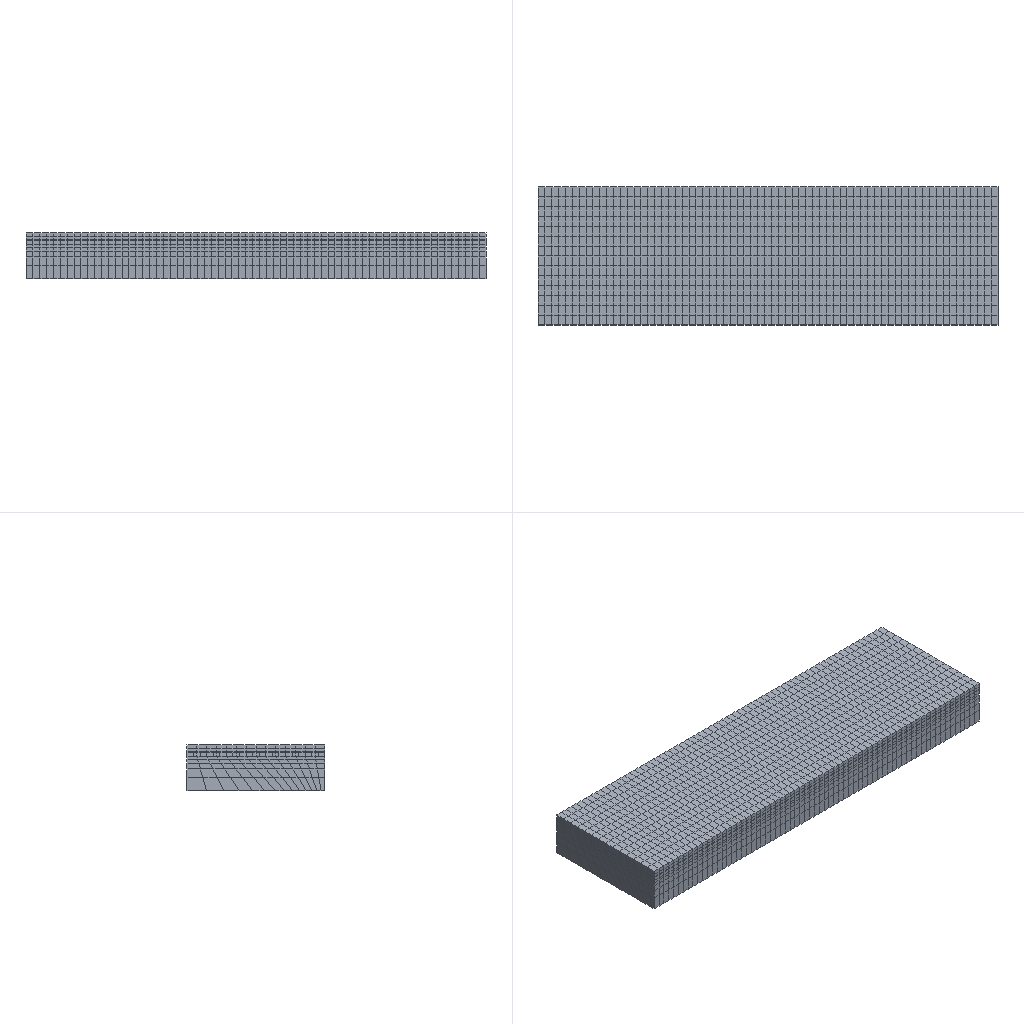Simulation study | abaqus
Set-up summary:
category,name,step,type,value,unit,region
solver,abaqus
solver,version,,,Abaqus/Explicit 2020
units,not stated in the deck,,not stated
analysis,deck,,transient,transient
load_step,Step-1,Step-1,transient
load_step,requested,,,1
mesh,nodes,,,12922
mesh,elements,,,9772
element_type,R3D3,,rigid,228
element_type,R3D4,,rigid,633
element_type,C3D8R,,solid,1407
element_type,EC3D8R,,solid,7504
load,load commands in deck,,count,1
bc,support commands in deck,,count,10
material,BING,,in results
material,WATER,,in results
check,setup vs results,,match,"per instance, exact: element labels, types and connectivity; labels of the nodes the elements use; coordinates of those nodes at SINGLE_PRECISION in 2 of 3 instance(s)"
Abaqus input file, long lists of numbers shortened:
*Heading
** Job name: Job-1 Model name: Model-1
** Generated by: Abaqus/CAE 2020
*Preprint, echo=NO, model=NO, history=NO, contact=NO
**
** PARTS
**
*Part, name=bing
*Node
      1,           0.,       -3000.,         900.
      2,       10000.,       -3000.,         900.
** (2990 more lines like these left out)
*Element, type=C3D8R
  1,  292,  617, 1013,  281,    1,   17,  148,    4
  2,  617,  618, 1014, 1013,   17,   18,  147,  148
** (1405 more lines like these left out)
*Nset, nset=Set-1, generate
    1,  2992,     1
*Elset, elset=Set-1, generate
    1,  1407,     1
** Section: bing
*Solid Section, elset=Set-1, material=bing
,
*End Part
**
*Part, name=oula
*Node
      1,       10000.,           0.,         750.
      2,       10000.,       -3000.,         750.
** (9178 more lines like these left out)
*Element, type=EC3D8R
   1,  212, 1143, 4033,  615,    1,   13,  511,   46
   2, 1143, 1144, 4034, 4033,   13,   14,  512,  511
** (7502 more lines like these left out)
*Nset, nset=Set-1, generate
    1,  9180,     1
*Elset, elset=Set-1, generate
    1,  7504,     1
** Section: oula
*Eulerian Section, elset=Set-1
water, water-1
*Surface, type=EULERIAN MATERIAL, name=water-1
water-1
*End Part
**
*Part, name=work
*Node
      1,    2.375,   6757.633,   37190.746
      2,    2.375,   6757.633,   40618.258
** (747 more lines like these left out)
*Element, type=R3D4
 1,  1, 21, 64,  4
 2, 21, 22, 63, 64
** (631 more lines like these left out)
*Element, type=R3D3
369,  4, 65,  5
370, 71, 59, 58
** (226 more lines like these left out)
*Node
    750,    2.375,   6959.508,   38910.039
*Nset, nset=work-RefPt_, internal
750,
*Elset, elset=work, generate
   1,  861,    1
*End Part
**
**
** ASSEMBLY
**
*Assembly, name=Assembly
**
*Instance, name=work-1, part=work
37076.822, -1497.625, -5616.383
37076.822, -1497.625, -5616.383, 37077.399, -1498.203, -5616.96,         120.
*End Instance
**
*Instance, name=oula-1, part=oula
          0.,           0.,         250.
*End Instance
**
*Instance, name=bing-1, part=bing
          0.,           0.,         100.
*End Instance
**
*Nset, nset=Set-1, instance=oula-1
    1,    2,    3,    4,    5,    6,    7,    8,   13,   14,   15,   16,   17,   18,   19,   20
   21,   22,   23,   24,   25,   26,   27,   28,   29,   30,   31,   32,   33,   34,   35,   36
** (381 more lines like these left out)
*Elset, elset=Set-1, instance=oula-1, generate
    1,  4690,     1
*Nset, nset=Set-2, instance=bing-1
   1,   2,   3,   4,   5,   6,   9,  12,  13,  14,  15,  16,  17,  18,  19,  20
  21,  22,  23,  24,  25,  26,  27,  28,  29,  30,  31,  32,  33,  34,  35,  36
** (18 more lines like these left out)
*Elset, elset=Set-2, instance=bing-1
    1,    2,    3,    4,    5,    6,    7,    8,    9,   10,   11,   12,   13,   14,   15,   16
   17,   18,   19,   20,   21,   22,   23,   24,   25,   26,   27,   28,   29,   30,   31,   32
** (8 more lines like these left out)
*Nset, nset=Set-3, instance=oula-1
    1,    2,    3,    4,    5,    6,    7,    8,    9,   10,   11,   12,   26,   27,   28,   29
   43,   44,   45,   46,   60,   61,   62,   63,   77,   78,   79,   80,   81,   82,   83,   84
** (75 more lines like these left out)
*Elset, elset=Set-3, instance=oula-1
    1,   14,   15,   28,   29,   42,   43,   56,   57,   70,   71,   84,   85,   98,   99,  112
  113,  126,  127,  140,  141,  154,  155,  168,  169,  182,  183,  196,  197,  210,  211,  224
** (65 more lines like these left out)
*Nset, nset=Set-4, instance=oula-1
    3,    4,    6,    7,   30,   31,   32,   33,   34,   35,   36,   37,   38,   39,   40,   41
   42,   64,   65,   66,   67,   68,   69,   70,   71,   72,   73,   74,   75,   76,   81,   82
** (62 more lines like these left out)
*Elset, elset=Set-4, instance=oula-1
   57,   58,   59,   60,   61,   62,   63,   64,   65,   66,   67,   68,   69,   70,  127,  128
  129,  130,  131,  132,  133,  134,  135,  136,  137,  138,  139,  140,  197,  198,  199,  200
** (57 more lines like these left out)
*Nset, nset=Set-5, instance=oula-1
   1,   2,   3,   4,  13,  14,  15,  16,  17,  18,  19,  20,  21,  22,  23,  24
  25,  26,  27,  28,  29,  30,  31,  32,  33,  34,  35,  36,  37,  38,  39,  40
** (4 more lines like these left out)
*Elset, elset=Set-5, instance=oula-1, generate
  1,  70,   1
*Nset, nset=Set-6, instance=work-1
 750,
*Rigid Body, ref node=work-1.work-RefPt_, elset=work-1.work
*End Assembly
**
** MATERIALS
**
*Material, name=bing
*Brittle Cracking
100.,  0.
250., 0.1
*Brittle Shear
1.,  0.
0., 0.1
*Brittle Failure
1.,
*Density
 9.2e-10,
*Elastic
1000., 0.3
*Material, name=water
*Density
 1e-09,
*Eos, type=USUP
1483.,0.,0.
*Viscosity
 0.01,
**
** INTERACTION PROPERTIES
**
*Surface Interaction, name=IntProp-1
*Friction
 0.2,
*Surface Behavior, pressure-overclosure=HARD
**
** PREDEFINED FIELDS
**
** Name: Predefined Field-1   Type: Material assignment
*Initial Conditions, type=VOLUME FRACTION
Set-1, oula-1.water-1, 1.
** ----------------------------------------------------------------
**
** STEP: Step-1
**
*Step, name=Step-1, nlgeom=YES
*Dynamic, Explicit
, 1.
*Bulk Viscosity
0.06, 1.2
** Mass Scaling: Semi-Automatic
**               Whole Model
*Fixed Mass Scaling, factor=5000.
**
** BOUNDARY CONDITIONS
**
** Name: BC-1 Type: 对称/反对称/完全固定
*Boundary
Set-2, ENCASTRE
** Name: [REDACTED] : Velocity/Angular velocity
*Boundary, type=VELOCITY
Set-4, 3, 3
** Name: [REDACTED] : Velocity/Angular velocity
*Boundary, type=VELOCITY
Set-5, 1, 1
** Name: [REDACTED] : Velocity/Angular velocity
*Boundary, type=VELOCITY
Set-3, 2, 2
** Name: [REDACTED] : Velocity/Angular velocity
*Boundary, type=VELOCITY
Set-6, 1, 1, 8300.
Set-6, 2, 2
Set-6, 3, 3
Set-6, 4, 4
Set-6, 5, 5
Set-6, 6, 6
**
** INTERACTIONS
**
** Interaction: Int-1
*Contact, op=NEW
*Contact Inclusions, ALL EXTERIOR
*Contact Property Assignment
 ,  , IntProp-1
**
** OUTPUT REQUESTS
**
*Restart, write, number interval=1, time marks=NO
**
** FIELD OUTPUT: F-Output-1
**
*Output, field, number interval=50
*Node Output
A, CF, RF, RM, RT, U, V
*Element Output, directions=YES
DENSITYVAVG, E, EVF, EVOL, LE, MISES, MISESMAX, PE, PEEQ, PEEQVAVG, PEVAVG, S, SF, SSAVG, STATUS, SVAVG
SVOL, TSHR
*Contact Output
CDISP, CSTRESS
**
** HISTORY OUTPUT: H-Output-1
**
*Output, history, time interval=5e-05
*Node Output, nset=Set-6
RF1, RF2, RF3
*End Step
Results summary:
result,step,Step-1,partial,increments=3050 time=0.1579/1.0
result,analysis,,,transient
result,last_loadstep,,,1
result,primary field,,,U
result,reaction total,,FX,2815175396.345,model units
result,reaction total,,FY,908360824.678,model units
result,reaction total,,FZ,179164417.669,model units